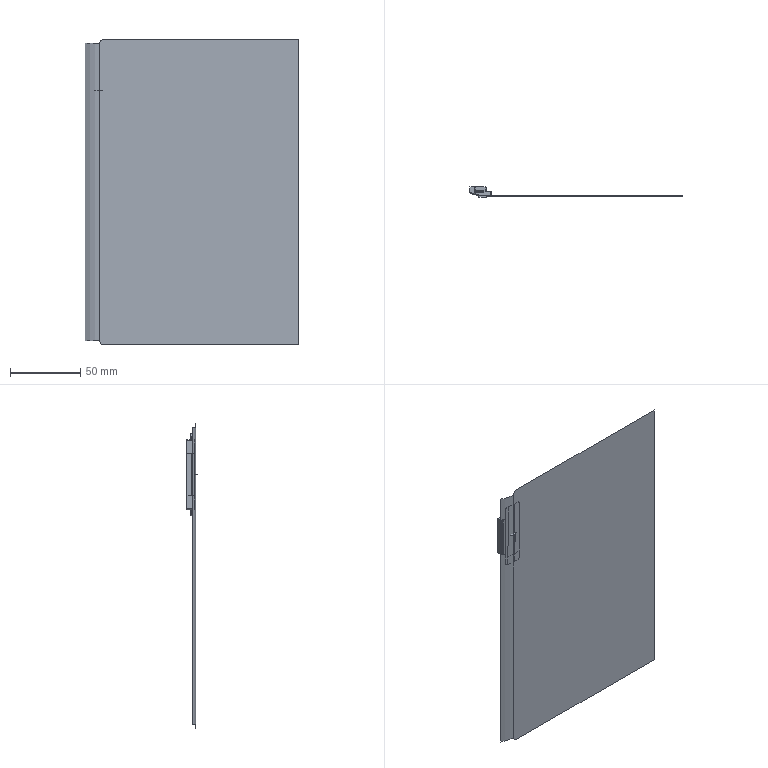Part | Creo | 1 solid | 52 faces | box 152.07 x 7.3 x 217.3 mm | volume 28108 mm3 | plane 28 | cylinder 17 | other 5 | spline 2 | commonest cylinder face diameters 2 x5 1.6 x4 3.5 x4 4.7 x2 1 x1 8 x1